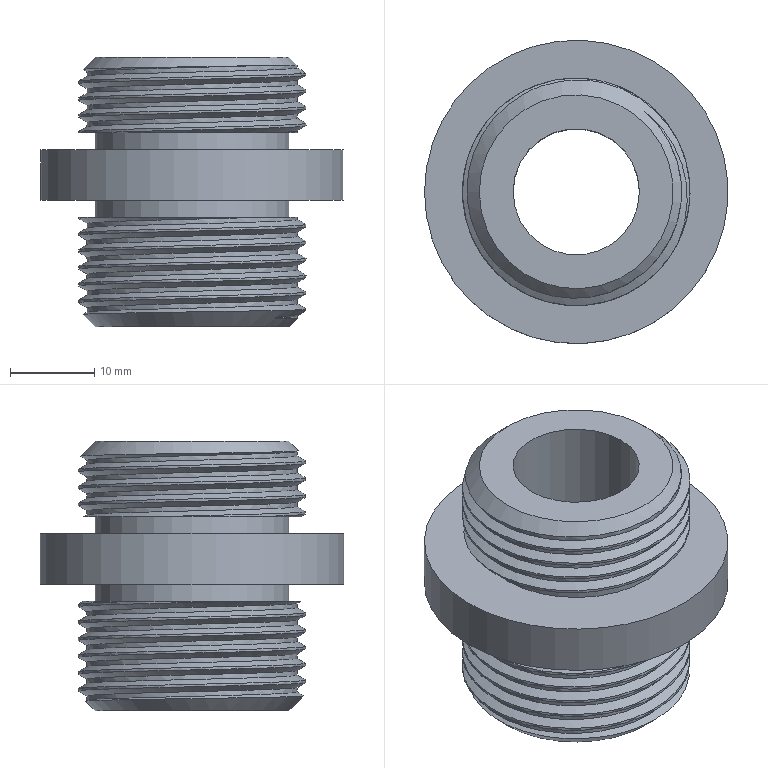Part | NX | features BREP 1, DATUM_CSYS 1 | 1 solid | 21 faces | box 36 x 36 x 32 mm | volume 13512 mm3 | cylinder 8 | plane 7 | spline 4 | cone 2 | commonest cylinder face diameters 23 x2 25 x2 27 x2 15 x1 36 x1